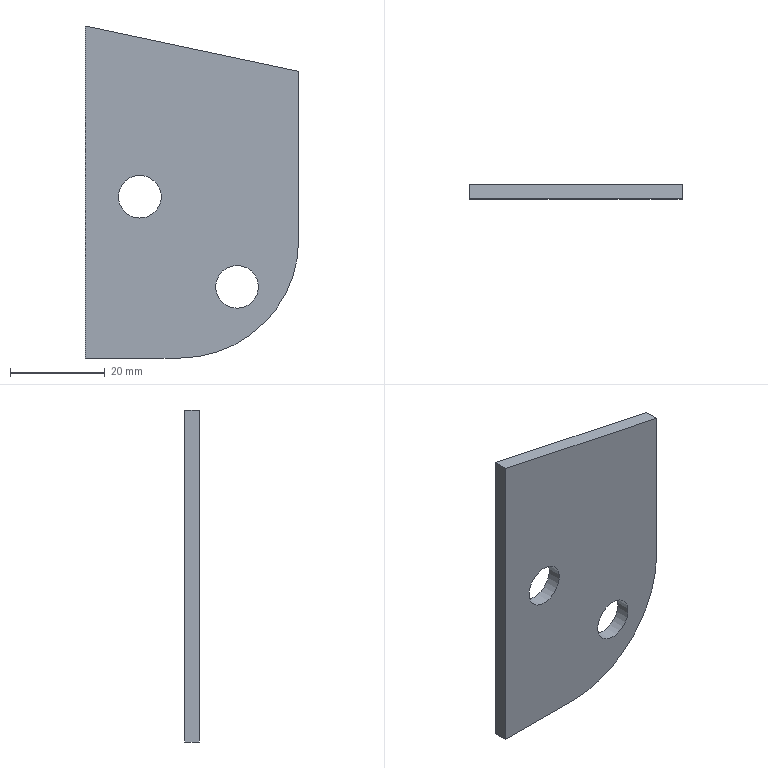Part | STEP file | 5091203 | 1 solid | 9 faces | box 45 x 3 x 70 mm | volume 8020 mm3 | plane 6 | cylinder 3 | commonest cylinder face diameters 9 x2 50 x1
STEP:
#1=CARTESIAN_POINT('',(0.,0.,0.));
#2=DIRECTION('',(0.,0.,1.));
#3=DIRECTION('',(1.,0.,0.));
#4=AXIS2_PLACEMENT_3D('',#1,#2,#3);
#5=CARTESIAN_POINT('',(22.5,1.5,25.435));
#6=VERTEX_POINT('',#5);
#7=CARTESIAN_POINT('',(22.5,1.5,-10.));
#8=VERTEX_POINT('',#7);
#9=CARTESIAN_POINT('',(22.5,1.5,35.));
#10=DIRECTION('',(0.,0.,-1.));
#11=VECTOR('',#10,1.);
#12=LINE('',#9,#11);
#13=CARTESIAN_POINT('',(22.5,1.5,35.));
#14=DIRECTION('',(-1.,0.,0.));
#15=DIRECTION('',(0.,0.,1.));
#16=AXIS2_PLACEMENT_3D('',#13,#14,#15);
#17=PLANE('',#16);
#18=CARTESIAN_POINT('',(0.,0.));
#19=DIRECTION('',(-1.,0.));
#20=VECTOR('',#19,1.);
#21=LINE('',#18,#20);
#22=(GEOMETRIC_REPRESENTATION_CONTEXT(2)PARAMETRIC_REPRESENTATION_CONTEXT()REPRESENTATION_CONTEXT('',''));
#23=DEFINITIONAL_REPRESENTATION('',(#21),#22);
#24=PCURVE('',#17,#23);
#25=CARTESIAN_POINT('',(-22.5,1.5,35.));
#26=DIRECTION('',(0.,-1.,0.));
#27=DIRECTION('',(0.,0.,-1.));
#28=AXIS2_PLACEMENT_3D('',#25,#26,#27);
#29=PLANE('',#28);
#30=CARTESIAN_POINT('',(0.,45.));
#31=DIRECTION('',(1.,0.));
#32=VECTOR('',#31,1.);
#33=LINE('',#30,#32);
#34=(GEOMETRIC_REPRESENTATION_CONTEXT(2)PARAMETRIC_REPRESENTATION_CONTEXT()REPRESENTATION_CONTEXT('',''));
#35=DEFINITIONAL_REPRESENTATION('',(#33),#34);
#36=PCURVE('',#29,#35);
#37=SURFACE_CURVE('',#12,(#24,#36),.PCURVE_S1.);
#38=EDGE_CURVE('',#6,#8,#37,.T.);
#39=ORIENTED_EDGE('',*,*,#38,.F.);
#40=CARTESIAN_POINT('',(22.5,-1.5,25.435));
#41=VERTEX_POINT('',#40);
#42=CARTESIAN_POINT('',(22.5,1.5,25.435));
#43=DIRECTION('',(0.,-1.,0.));
#44=VECTOR('',#43,1.);
#45=LINE('',#42,#44);
#46=CARTESIAN_POINT('',(-9.565,0.));
#47=DIRECTION('',(0.,-1.));
#48=VECTOR('',#47,1.);
#49=LINE('',#46,#48);
#50=(GEOMETRIC_REPRESENTATION_CONTEXT(2)PARAMETRIC_REPRESENTATION_CONTEXT()REPRESENTATION_CONTEXT('',''));
#51=DEFINITIONAL_REPRESENTATION('',(#49),#50);
#52=PCURVE('',#17,#51);
#53=CARTESIAN_POINT('',(-22.5,109.338,35.));
#54=DIRECTION('',(-0.2079,0.,-0.9781));
#55=DIRECTION('',(-0.9781,0.,0.2079));
#56=AXIS2_PLACEMENT_3D('',#53,#54,#55);
#57=PLANE('',#56);
#58=CARTESIAN_POINT('',(-46.005,-107.838));
#59=DIRECTION('',(0.,-1.));
#60=VECTOR('',#59,1.);
#61=LINE('',#58,#60);
#62=(GEOMETRIC_REPRESENTATION_CONTEXT(2)PARAMETRIC_REPRESENTATION_CONTEXT()REPRESENTATION_CONTEXT('',''));
#63=DEFINITIONAL_REPRESENTATION('',(#61),#62);
#64=PCURVE('',#57,#63);
#65=SURFACE_CURVE('',#45,(#52,#64),.PCURVE_S1.);
#66=EDGE_CURVE('',#6,#41,#65,.T.);
#67=ORIENTED_EDGE('',*,*,#66,.T.);
#68=CARTESIAN_POINT('',(22.5,-1.5,-10.));
#69=VERTEX_POINT('',#68);
#70=CARTESIAN_POINT('',(22.5,-1.5,35.));
#71=DIRECTION('',(0.,0.,-1.));
#72=VECTOR('',#71,1.);
#73=LINE('',#70,#72);
#74=CARTESIAN_POINT('',(0.,-3.));
#75=DIRECTION('',(-1.,0.));
#76=VECTOR('',#75,1.);
#77=LINE('',#74,#76);
#78=(GEOMETRIC_REPRESENTATION_CONTEXT(2)PARAMETRIC_REPRESENTATION_CONTEXT()REPRESENTATION_CONTEXT('',''));
#79=DEFINITIONAL_REPRESENTATION('',(#77),#78);
#80=PCURVE('',#17,#79);
#81=CARTESIAN_POINT('',(-22.5,-1.5,35.));
#82=DIRECTION('',(0.,1.,0.));
#83=DIRECTION('',(0.,0.,1.));
#84=AXIS2_PLACEMENT_3D('',#81,#82,#83);
#85=PLANE('',#84);
#86=CARTESIAN_POINT('',(0.,45.));
#87=DIRECTION('',(-1.,0.));
#88=VECTOR('',#87,1.);
#89=LINE('',#86,#88);
#90=(GEOMETRIC_REPRESENTATION_CONTEXT(2)PARAMETRIC_REPRESENTATION_CONTEXT()REPRESENTATION_CONTEXT('',''));
#91=DEFINITIONAL_REPRESENTATION('',(#89),#90);
#92=PCURVE('',#85,#91);
#93=SURFACE_CURVE('',#73,(#80,#92),.PCURVE_S1.);
#94=EDGE_CURVE('',#41,#69,#93,.T.);
#95=ORIENTED_EDGE('',*,*,#94,.T.);
#96=CARTESIAN_POINT('',(22.5,1.5,-10.));
#97=DIRECTION('',(0.,1.,0.));
#98=VECTOR('',#97,1.);
#99=LINE('',#96,#98);
#100=CARTESIAN_POINT('',(-45.,0.));
#101=DIRECTION('',(0.,1.));
#102=VECTOR('',#101,1.);
#103=LINE('',#100,#102);
#104=(GEOMETRIC_REPRESENTATION_CONTEXT(2)PARAMETRIC_REPRESENTATION_CONTEXT()REPRESENTATION_CONTEXT('',''));
#105=DEFINITIONAL_REPRESENTATION('',(#103),#104);
#106=PCURVE('',#17,#105);
#107=CARTESIAN_POINT('',(-2.5,1.5,-10.));
#108=DIRECTION('',(0.,1.,0.));
#109=DIRECTION('',(0.,0.,1.));
#110=AXIS2_PLACEMENT_3D('',#107,#108,#109);
#111=CYLINDRICAL_SURFACE('',#110,25.);
#112=CARTESIAN_POINT('',(1.571,0.));
#113=DIRECTION('',(0.,1.));
#114=VECTOR('',#113,1.);
#115=LINE('',#112,#114);
#116=(GEOMETRIC_REPRESENTATION_CONTEXT(2)PARAMETRIC_REPRESENTATION_CONTEXT()REPRESENTATION_CONTEXT('',''));
#117=DEFINITIONAL_REPRESENTATION('',(#115),#116);
#118=PCURVE('',#111,#117);
#119=SURFACE_CURVE('',#99,(#106,#118),.PCURVE_S1.);
#120=EDGE_CURVE('',#69,#8,#119,.T.);
#121=ORIENTED_EDGE('',*,*,#120,.T.);
#122=EDGE_LOOP('',(#39,#67,#95,#121));
#123=FACE_BOUND('',#122,.T.);
#124=ADVANCED_FACE('',(#123),#17,.F.);
#125=CARTESIAN_POINT('',(9.5,1.5,-15.5));
#126=VERTEX_POINT('',#125);
#127=CARTESIAN_POINT('',(9.5,1.5,-20.));
#128=DIRECTION('',(0.,1.,0.));
#129=DIRECTION('',(0.,0.,1.));
#130=AXIS2_PLACEMENT_3D('',#127,#128,#129);
#131=CIRCLE('',#130,4.5);
#132=CARTESIAN_POINT('',(50.5,32.));
#133=CARTESIAN_POINT('',(50.5,39.794));
#134=CARTESIAN_POINT('',(57.25,35.897));
#135=CARTESIAN_POINT('',(64.,32.));
#136=CARTESIAN_POINT('',(57.25,28.103));
#137=CARTESIAN_POINT('',(50.5,24.206));
#138=CARTESIAN_POINT('',(50.5,32.));
#139=(BOUNDED_CURVE()B_SPLINE_CURVE(2,(#132,#133,#134,#135,#136,#137,#138),.UNSPECIFIED.,.T.,.F.)B_SPLINE_CURVE_WITH_KNOTS((1,2,2,2,2,1),(-2.094,0.,2.094,4.189,6.283,8.378),.UNSPECIFIED.)CURVE()GEOMETRIC_REPRESENTATION_ITEM()RATIONAL_B_SPLINE_CURVE((1.,0.5,1.,0.5,1.,0.5,1.))REPRESENTATION_ITEM(''));
#140=(GEOMETRIC_REPRESENTATION_CONTEXT(2)PARAMETRIC_REPRESENTATION_CONTEXT()REPRESENTATION_CONTEXT('',''));
#141=DEFINITIONAL_REPRESENTATION('',(#139),#140);
#142=PCURVE('',#29,#141);
#143=CARTESIAN_POINT('',(9.5,-8.5,-20.));
#144=DIRECTION('',(0.,1.,0.));
#145=DIRECTION('',(0.,0.,1.));
#146=AXIS2_PLACEMENT_3D('',#143,#144,#145);
#147=CYLINDRICAL_SURFACE('',#146,4.5);
#148=CARTESIAN_POINT('',(0.,10.));
#149=DIRECTION('',(1.,0.));
#150=VECTOR('',#149,1.);
#151=LINE('',#148,#150);
#152=(GEOMETRIC_REPRESENTATION_CONTEXT(2)PARAMETRIC_REPRESENTATION_CONTEXT()REPRESENTATION_CONTEXT('',''));
#153=DEFINITIONAL_REPRESENTATION('',(#151),#152);
#154=PCURVE('',#147,#153);
#155=SURFACE_CURVE('',#131,(#142,#154),.PCURVE_S1.);
#156=EDGE_CURVE('',#126,#126,#155,.T.);
#157=ORIENTED_EDGE('',*,*,#156,.F.);
#158=EDGE_LOOP('',(#157));
#159=FACE_BOUND('',#158,.T.);
#160=CARTESIAN_POINT('',(-11.,1.5,3.5));
#161=VERTEX_POINT('',#160);
#162=CARTESIAN_POINT('',(-11.,1.5,-1.));
#163=DIRECTION('',(0.,1.,0.));
#164=DIRECTION('',(0.,0.,1.));
#165=AXIS2_PLACEMENT_3D('',#162,#163,#164);
#166=CIRCLE('',#165,4.5);
#167=CARTESIAN_POINT('',(31.5,11.5));
#168=CARTESIAN_POINT('',(31.5,19.294));
#169=CARTESIAN_POINT('',(38.25,15.397));
#170=CARTESIAN_POINT('',(45.,11.5));
#171=CARTESIAN_POINT('',(38.25,7.603));
#172=CARTESIAN_POINT('',(31.5,3.706));
#173=CARTESIAN_POINT('',(31.5,11.5));
#174=(BOUNDED_CURVE()B_SPLINE_CURVE(2,(#167,#168,#169,#170,#171,#172,#173),.UNSPECIFIED.,.T.,.F.)B_SPLINE_CURVE_WITH_KNOTS((1,2,2,2,2,1),(-2.094,0.,2.094,4.189,6.283,8.378),.UNSPECIFIED.)CURVE()GEOMETRIC_REPRESENTATION_ITEM()RATIONAL_B_SPLINE_CURVE((1.,0.5,1.,0.5,1.,0.5,1.))REPRESENTATION_ITEM(''));
#175=(GEOMETRIC_REPRESENTATION_CONTEXT(2)PARAMETRIC_REPRESENTATION_CONTEXT()REPRESENTATION_CONTEXT('',''));
#176=DEFINITIONAL_REPRESENTATION('',(#174),#175);
#177=PCURVE('',#29,#176);
#178=CARTESIAN_POINT('',(-11.,-8.5,-1.));
#179=DIRECTION('',(0.,1.,0.));
#180=DIRECTION('',(0.,0.,1.));
#181=AXIS2_PLACEMENT_3D('',#178,#179,#180);
#182=CYLINDRICAL_SURFACE('',#181,4.5);
#183=CARTESIAN_POINT('',(0.,10.));
#184=DIRECTION('',(1.,0.));
#185=VECTOR('',#184,1.);
#186=LINE('',#183,#185);
#187=(GEOMETRIC_REPRESENTATION_CONTEXT(2)PARAMETRIC_REPRESENTATION_CONTEXT()REPRESENTATION_CONTEXT('',''));
#188=DEFINITIONAL_REPRESENTATION('',(#186),#187);
#189=PCURVE('',#182,#188);
#190=SURFACE_CURVE('',#166,(#177,#189),.PCURVE_S1.);
#191=EDGE_CURVE('',#161,#161,#190,.T.);
#192=ORIENTED_EDGE('',*,*,#191,.F.);
#193=EDGE_LOOP('',(#192));
#194=FACE_BOUND('',#193,.T.);
#195=CARTESIAN_POINT('',(-22.5,1.5,35.));
#196=VERTEX_POINT('',#195);
#197=CARTESIAN_POINT('',(-22.5,1.5,-35.));
#198=VERTEX_POINT('',#197);
#199=CARTESIAN_POINT('',(-22.5,1.5,35.));
#200=DIRECTION('',(0.,0.,-1.));
#201=VECTOR('',#200,1.);
#202=LINE('',#199,#201);
#203=CARTESIAN_POINT('',(0.,0.));
#204=DIRECTION('',(1.,0.));
#205=VECTOR('',#204,1.);
#206=LINE('',#203,#205);
#207=(GEOMETRIC_REPRESENTATION_CONTEXT(2)PARAMETRIC_REPRESENTATION_CONTEXT()REPRESENTATION_CONTEXT('',''));
#208=DEFINITIONAL_REPRESENTATION('',(#206),#207);
#209=PCURVE('',#29,#208);
#210=CARTESIAN_POINT('',(-22.5,1.5,35.));
#211=DIRECTION('',(1.,0.,0.));
#212=DIRECTION('',(0.,0.,-1.));
#213=AXIS2_PLACEMENT_3D('',#210,#211,#212);
#214=PLANE('',#213);
#215=CARTESIAN_POINT('',(0.,0.));
#216=DIRECTION('',(1.,0.));
#217=VECTOR('',#216,1.);
#218=LINE('',#215,#217);
#219=(GEOMETRIC_REPRESENTATION_CONTEXT(2)PARAMETRIC_REPRESENTATION_CONTEXT()REPRESENTATION_CONTEXT('',''));
#220=DEFINITIONAL_REPRESENTATION('',(#218),#219);
#221=PCURVE('',#214,#220);
#222=SURFACE_CURVE('',#202,(#209,#221),.PCURVE_S1.);
#223=EDGE_CURVE('',#196,#198,#222,.T.);
#224=ORIENTED_EDGE('',*,*,#223,.F.);
#225=CARTESIAN_POINT('',(-22.5,1.5,35.));
#226=DIRECTION('',(0.9781,0.,-0.2079));
#227=VECTOR('',#226,1.);
#228=LINE('',#225,#227);
#229=CARTESIAN_POINT('',(0.,0.));
#230=DIRECTION('',(0.2079,0.9781));
#231=VECTOR('',#230,1.);
#232=LINE('',#229,#231);
#233=(GEOMETRIC_REPRESENTATION_CONTEXT(2)PARAMETRIC_REPRESENTATION_CONTEXT()REPRESENTATION_CONTEXT('',''));
#234=DEFINITIONAL_REPRESENTATION('',(#232),#233);
#235=PCURVE('',#29,#234);
#236=CARTESIAN_POINT('',(0.,-107.838));
#237=DIRECTION('',(-1.,0.));
#238=VECTOR('',#237,1.);
#239=LINE('',#236,#238);
#240=(GEOMETRIC_REPRESENTATION_CONTEXT(2)PARAMETRIC_REPRESENTATION_CONTEXT()REPRESENTATION_CONTEXT('',''));
#241=DEFINITIONAL_REPRESENTATION('',(#239),#240);
#242=PCURVE('',#57,#241);
#243=SURFACE_CURVE('',#228,(#235,#242),.PCURVE_S1.);
#244=EDGE_CURVE('',#196,#6,#243,.T.);
#245=ORIENTED_EDGE('',*,*,#244,.T.);
#246=ORIENTED_EDGE('',*,*,#38,.T.);
#247=CARTESIAN_POINT('',(-2.5,1.5,-35.));
#248=VERTEX_POINT('',#247);
#249=CARTESIAN_POINT('',(-2.5,1.5,-10.));
#250=DIRECTION('',(0.,1.,0.));
#251=DIRECTION('',(0.,0.,-1.));
#252=AXIS2_PLACEMENT_3D('',#249,#250,#251);
#253=CIRCLE('',#252,25.);
#254=CARTESIAN_POINT('',(70.,20.));
#255=CARTESIAN_POINT('',(70.,-23.301));
#256=CARTESIAN_POINT('',(32.5,-1.651));
#257=CARTESIAN_POINT('',(-5.,20.));
#258=CARTESIAN_POINT('',(32.5,41.651));
#259=CARTESIAN_POINT('',(70.,63.301));
#260=CARTESIAN_POINT('',(70.,20.));
#261=(BOUNDED_CURVE()B_SPLINE_CURVE(2,(#254,#255,#256,#257,#258,#259,#260),.UNSPECIFIED.,.T.,.F.)B_SPLINE_CURVE_WITH_KNOTS((1,2,2,2,2,1),(-2.094,0.,2.094,4.189,6.283,8.378),.UNSPECIFIED.)CURVE()GEOMETRIC_REPRESENTATION_ITEM()RATIONAL_B_SPLINE_CURVE((1.,0.5,1.,0.5,1.,0.5,1.))REPRESENTATION_ITEM(''));
#262=(GEOMETRIC_REPRESENTATION_CONTEXT(2)PARAMETRIC_REPRESENTATION_CONTEXT()REPRESENTATION_CONTEXT('',''));
#263=DEFINITIONAL_REPRESENTATION('',(#261),#262);
#264=PCURVE('',#29,#263);
#265=CARTESIAN_POINT('',(-3.142,0.));
#266=DIRECTION('',(1.,0.));
#267=VECTOR('',#266,1.);
#268=LINE('',#265,#267);
#269=(GEOMETRIC_REPRESENTATION_CONTEXT(2)PARAMETRIC_REPRESENTATION_CONTEXT()REPRESENTATION_CONTEXT('',''));
#270=DEFINITIONAL_REPRESENTATION('',(#268),#269);
#271=PCURVE('',#111,#270);
#272=SURFACE_CURVE('',#253,(#264,#271),.PCURVE_S1.);
#273=EDGE_CURVE('',#8,#248,#272,.T.);
#274=ORIENTED_EDGE('',*,*,#273,.T.);
#275=CARTESIAN_POINT('',(-22.5,1.5,-35.));
#276=DIRECTION('',(-1.,0.,0.));
#277=VECTOR('',#276,1.);
#278=LINE('',#275,#277);
#279=CARTESIAN_POINT('',(70.,0.));
#280=DIRECTION('',(0.,-1.));
#281=VECTOR('',#280,1.);
#282=LINE('',#279,#281);
#283=(GEOMETRIC_REPRESENTATION_CONTEXT(2)PARAMETRIC_REPRESENTATION_CONTEXT()REPRESENTATION_CONTEXT('',''));
#284=DEFINITIONAL_REPRESENTATION('',(#282),#283);
#285=PCURVE('',#29,#284);
#286=CARTESIAN_POINT('',(0.,0.,-35.));
#287=DIRECTION('',(0.,0.,1.));
#288=DIRECTION('',(1.,0.,0.));
#289=AXIS2_PLACEMENT_3D('',#286,#287,#288);
#290=PLANE('',#289);
#291=CARTESIAN_POINT('',(-22.5,1.5));
#292=DIRECTION('',(-1.,0.));
#293=VECTOR('',#292,1.);
#294=LINE('',#291,#293);
#295=(GEOMETRIC_REPRESENTATION_CONTEXT(2)PARAMETRIC_REPRESENTATION_CONTEXT()REPRESENTATION_CONTEXT('',''));
#296=DEFINITIONAL_REPRESENTATION('',(#294),#295);
#297=PCURVE('',#290,#296);
#298=SURFACE_CURVE('',#278,(#285,#297),.PCURVE_S1.);
#299=EDGE_CURVE('',#248,#198,#298,.T.);
#300=ORIENTED_EDGE('',*,*,#299,.T.);
#301=EDGE_LOOP('',(#224,#245,#246,#274,#300));
#302=FACE_BOUND('',#301,.T.);
#303=ADVANCED_FACE('',(#159,#194,#302),#29,.F.);
#304=CARTESIAN_POINT('',(-22.5,-1.5,-35.));
#305=VERTEX_POINT('',#304);
#306=CARTESIAN_POINT('',(-22.5,1.5,-35.));
#307=DIRECTION('',(0.,-1.,0.));
#308=VECTOR('',#307,1.);
#309=LINE('',#306,#308);
#310=CARTESIAN_POINT('',(70.,0.));
#311=DIRECTION('',(0.,-1.));
#312=VECTOR('',#311,1.);
#313=LINE('',#310,#312);
#314=(GEOMETRIC_REPRESENTATION_CONTEXT(2)PARAMETRIC_REPRESENTATION_CONTEXT()REPRESENTATION_CONTEXT('',''));
#315=DEFINITIONAL_REPRESENTATION('',(#313),#314);
#316=PCURVE('',#214,#315);
#317=CARTESIAN_POINT('',(-22.5,1.5));
#318=DIRECTION('',(0.,-1.));
#319=VECTOR('',#318,1.);
#320=LINE('',#317,#319);
#321=(GEOMETRIC_REPRESENTATION_CONTEXT(2)PARAMETRIC_REPRESENTATION_CONTEXT()REPRESENTATION_CONTEXT('',''));
#322=DEFINITIONAL_REPRESENTATION('',(#320),#321);
#323=PCURVE('',#290,#322);
#324=SURFACE_CURVE('',#309,(#316,#323),.PCURVE_S1.);
#325=EDGE_CURVE('',#198,#305,#324,.T.);
#326=ORIENTED_EDGE('',*,*,#325,.T.);
#327=CARTESIAN_POINT('',(-22.5,-1.5,35.));
#328=VERTEX_POINT('',#327);
#329=CARTESIAN_POINT('',(-22.5,-1.5,35.));
#330=DIRECTION('',(0.,0.,-1.));
#331=VECTOR('',#330,1.);
#332=LINE('',#329,#331);
#333=CARTESIAN_POINT('',(0.,-3.));
#334=DIRECTION('',(1.,0.));
#335=VECTOR('',#334,1.);
#336=LINE('',#333,#335);
#337=(GEOMETRIC_REPRESENTATION_CONTEXT(2)PARAMETRIC_REPRESENTATION_CONTEXT()REPRESENTATION_CONTEXT('',''));
#338=DEFINITIONAL_REPRESENTATION('',(#336),#337);
#339=PCURVE('',#214,#338);
#340=CARTESIAN_POINT('',(0.,0.));
#341=DIRECTION('',(-1.,0.));
#342=VECTOR('',#341,1.);
#343=LINE('',#340,#342);
#344=(GEOMETRIC_REPRESENTATION_CONTEXT(2)PARAMETRIC_REPRESENTATION_CONTEXT()REPRESENTATION_CONTEXT('',''));
#345=DEFINITIONAL_REPRESENTATION('',(#343),#344);
#346=PCURVE('',#85,#345);
#347=SURFACE_CURVE('',#332,(#339,#346),.PCURVE_S1.);
#348=EDGE_CURVE('',#328,#305,#347,.T.);
#349=ORIENTED_EDGE('',*,*,#348,.F.);
#350=CARTESIAN_POINT('',(-22.5,1.5,35.));
#351=DIRECTION('',(0.,-1.,0.));
#352=VECTOR('',#351,1.);
#353=LINE('',#350,#352);
#354=CARTESIAN_POINT('',(0.,0.));
#355=DIRECTION('',(0.,-1.));
#356=VECTOR('',#355,1.);
#357=LINE('',#354,#356);
#358=(GEOMETRIC_REPRESENTATION_CONTEXT(2)PARAMETRIC_REPRESENTATION_CONTEXT()REPRESENTATION_CONTEXT('',''));
#359=DEFINITIONAL_REPRESENTATION('',(#357),#358);
#360=PCURVE('',#214,#359);
#361=CARTESIAN_POINT('',(0.,-107.838));
#362=DIRECTION('',(0.,-1.));
#363=VECTOR('',#362,1.);
#364=LINE('',#361,#363);
#365=(GEOMETRIC_REPRESENTATION_CONTEXT(2)PARAMETRIC_REPRESENTATION_CONTEXT()REPRESENTATION_CONTEXT('',''));
#366=DEFINITIONAL_REPRESENTATION('',(#364),#365);
#367=PCURVE('',#57,#366);
#368=SURFACE_CURVE('',#353,(#360,#367),.PCURVE_S1.);
#369=EDGE_CURVE('',#196,#328,#368,.T.);
#370=ORIENTED_EDGE('',*,*,#369,.F.);
#371=ORIENTED_EDGE('',*,*,#223,.T.);
#372=EDGE_LOOP('',(#326,#349,#370,#371));
#373=FACE_BOUND('',#372,.T.);
#374=ADVANCED_FACE('',(#373),#214,.F.);
#375=CARTESIAN_POINT('',(9.5,-1.5,-15.5));
#376=VERTEX_POINT('',#375);
#377=CARTESIAN_POINT('',(9.5,-1.5,-20.));
#378=DIRECTION('',(0.,1.,0.));
#379=DIRECTION('',(0.,0.,1.));
#380=AXIS2_PLACEMENT_3D('',#377,#378,#379);
#381=CIRCLE('',#380,4.5);
#382=CARTESIAN_POINT('',(-55.,32.));
#383=DIRECTION('',(1.,0.));
#384=AXIS2_PLACEMENT_2D('',#382,#383);
#385=CIRCLE('',#384,4.5);
#386=(GEOMETRIC_REPRESENTATION_CONTEXT(2)PARAMETRIC_REPRESENTATION_CONTEXT()REPRESENTATION_CONTEXT('',''));
#387=DEFINITIONAL_REPRESENTATION('',(#385),#386);
#388=PCURVE('',#85,#387);
#389=CARTESIAN_POINT('',(0.,7.));
#390=DIRECTION('',(1.,0.));
#391=VECTOR('',#390,1.);
#392=LINE('',#389,#391);
#393=(GEOMETRIC_REPRESENTATION_CONTEXT(2)PARAMETRIC_REPRESENTATION_CONTEXT()REPRESENTATION_CONTEXT('',''));
#394=DEFINITIONAL_REPRESENTATION('',(#392),#393);
#395=PCURVE('',#147,#394);
#396=SURFACE_CURVE('',#381,(#388,#395),.PCURVE_S1.);
#397=EDGE_CURVE('',#376,#376,#396,.T.);
#398=ORIENTED_EDGE('',*,*,#397,.T.);
#399=EDGE_LOOP('',(#398));
#400=FACE_BOUND('',#399,.T.);
#401=CARTESIAN_POINT('',(-11.,-1.5,3.5));
#402=VERTEX_POINT('',#401);
#403=CARTESIAN_POINT('',(-11.,-1.5,-1.));
#404=DIRECTION('',(0.,1.,0.));
#405=DIRECTION('',(0.,0.,1.));
#406=AXIS2_PLACEMENT_3D('',#403,#404,#405);
#407=CIRCLE('',#406,4.5);
#408=CARTESIAN_POINT('',(-36.,11.5));
#409=DIRECTION('',(1.,0.));
#410=AXIS2_PLACEMENT_2D('',#408,#409);
#411=CIRCLE('',#410,4.5);
#412=(GEOMETRIC_REPRESENTATION_CONTEXT(2)PARAMETRIC_REPRESENTATION_CONTEXT()REPRESENTATION_CONTEXT('',''));
#413=DEFINITIONAL_REPRESENTATION('',(#411),#412);
#414=PCURVE('',#85,#413);
#415=CARTESIAN_POINT('',(0.,7.));
#416=DIRECTION('',(1.,0.));
#417=VECTOR('',#416,1.);
#418=LINE('',#415,#417);
#419=(GEOMETRIC_REPRESENTATION_CONTEXT(2)PARAMETRIC_REPRESENTATION_CONTEXT()REPRESENTATION_CONTEXT('',''));
#420=DEFINITIONAL_REPRESENTATION('',(#418),#419);
#421=PCURVE('',#182,#420);
#422=SURFACE_CURVE('',#407,(#414,#421),.PCURVE_S1.);
#423=EDGE_CURVE('',#402,#402,#422,.T.);
#424=ORIENTED_EDGE('',*,*,#423,.T.);
#425=EDGE_LOOP('',(#424));
#426=FACE_BOUND('',#425,.T.);
#427=ORIENTED_EDGE('',*,*,#94,.F.);
#428=CARTESIAN_POINT('',(-22.5,-1.5,35.));
#429=DIRECTION('',(-0.9781,0.,0.2079));
#430=VECTOR('',#429,1.);
#431=LINE('',#428,#430);
#432=CARTESIAN_POINT('',(0.,0.));
#433=DIRECTION('',(0.2079,-0.9781));
#434=VECTOR('',#433,1.);
#435=LINE('',#432,#434);
#436=(GEOMETRIC_REPRESENTATION_CONTEXT(2)PARAMETRIC_REPRESENTATION_CONTEXT()REPRESENTATION_CONTEXT('',''));
#437=DEFINITIONAL_REPRESENTATION('',(#435),#436);
#438=PCURVE('',#85,#437);
#439=CARTESIAN_POINT('',(0.,-110.838));
#440=DIRECTION('',(1.,0.));
#441=VECTOR('',#440,1.);
#442=LINE('',#439,#441);
#443=(GEOMETRIC_REPRESENTATION_CONTEXT(2)PARAMETRIC_REPRESENTATION_CONTEXT()REPRESENTATION_CONTEXT('',''));
#444=DEFINITIONAL_REPRESENTATION('',(#442),#443);
#445=PCURVE('',#57,#444);
#446=SURFACE_CURVE('',#431,(#438,#445),.PCURVE_S1.);
#447=EDGE_CURVE('',#41,#328,#446,.T.);
#448=ORIENTED_EDGE('',*,*,#447,.T.);
#449=ORIENTED_EDGE('',*,*,#348,.T.);
#450=CARTESIAN_POINT('',(-2.5,-1.5,-35.));
#451=VERTEX_POINT('',#450);
#452=CARTESIAN_POINT('',(-22.5,-1.5,-35.));
#453=DIRECTION('',(1.,0.,0.));
#454=VECTOR('',#453,1.);
#455=LINE('',#452,#454);
#456=CARTESIAN_POINT('',(-70.,0.));
#457=DIRECTION('',(0.,1.));
#458=VECTOR('',#457,1.);
#459=LINE('',#456,#458);
#460=(GEOMETRIC_REPRESENTATION_CONTEXT(2)PARAMETRIC_REPRESENTATION_CONTEXT()REPRESENTATION_CONTEXT('',''));
#461=DEFINITIONAL_REPRESENTATION('',(#459),#460);
#462=PCURVE('',#85,#461);
#463=CARTESIAN_POINT('',(-22.5,-1.5));
#464=DIRECTION('',(1.,0.));
#465=VECTOR('',#464,1.);
#466=LINE('',#463,#465);
#467=(GEOMETRIC_REPRESENTATION_CONTEXT(2)PARAMETRIC_REPRESENTATION_CONTEXT()REPRESENTATION_CONTEXT('',''));
#468=DEFINITIONAL_REPRESENTATION('',(#466),#467);
#469=PCURVE('',#290,#468);
#470=SURFACE_CURVE('',#455,(#462,#469),.PCURVE_S1.);
#471=EDGE_CURVE('',#305,#451,#470,.T.);
#472=ORIENTED_EDGE('',*,*,#471,.T.);
#473=CARTESIAN_POINT('',(-2.5,-1.5,-10.));
#474=DIRECTION('',(0.,-1.,0.));
#475=DIRECTION('',(0.,0.,1.));
#476=AXIS2_PLACEMENT_3D('',#473,#474,#475);
#477=CIRCLE('',#476,25.);
#478=CARTESIAN_POINT('',(-20.,20.));
#479=CARTESIAN_POINT('',(-20.,-23.301));
#480=CARTESIAN_POINT('',(-57.5,-1.651));
#481=CARTESIAN_POINT('',(-95.,20.));
#482=CARTESIAN_POINT('',(-57.5,41.651));
#483=CARTESIAN_POINT('',(-20.,63.301));
#484=CARTESIAN_POINT('',(-20.,20.));
#485=(BOUNDED_CURVE()B_SPLINE_CURVE(2,(#478,#479,#480,#481,#482,#483,#484),.UNSPECIFIED.,.T.,.F.)B_SPLINE_CURVE_WITH_KNOTS((1,2,2,2,2,1),(-2.094,0.,2.094,4.189,6.283,8.378),.UNSPECIFIED.)CURVE()GEOMETRIC_REPRESENTATION_ITEM()RATIONAL_B_SPLINE_CURVE((1.,0.5,1.,0.5,1.,0.5,1.))REPRESENTATION_ITEM(''));
#486=(GEOMETRIC_REPRESENTATION_CONTEXT(2)PARAMETRIC_REPRESENTATION_CONTEXT()REPRESENTATION_CONTEXT('',''));
#487=DEFINITIONAL_REPRESENTATION('',(#485),#486);
#488=PCURVE('',#85,#487);
#489=CARTESIAN_POINT('',(6.283,-3.));
#490=DIRECTION('',(-1.,0.));
#491=VECTOR('',#490,1.);
#492=LINE('',#489,#491);
#493=(GEOMETRIC_REPRESENTATION_CONTEXT(2)PARAMETRIC_REPRESENTATION_CONTEXT()REPRESENTATION_CONTEXT('',''));
#494=DEFINITIONAL_REPRESENTATION('',(#492),#493);
#495=PCURVE('',#111,#494);
#496=SURFACE_CURVE('',#477,(#488,#495),.PCURVE_S1.);
#497=EDGE_CURVE('',#451,#69,#496,.T.);
#498=ORIENTED_EDGE('',*,*,#497,.T.);
#499=EDGE_LOOP('',(#427,#448,#449,#472,#498));
#500=FACE_BOUND('',#499,.T.);
#501=ADVANCED_FACE('',(#400,#426,#500),#85,.F.);
#502=ORIENTED_EDGE('',*,*,#299,.F.);
#503=CARTESIAN_POINT('',(-2.5,0.,-35.));
#504=DIRECTION('',(0.,-1.,0.));
#505=VECTOR('',#504,1.);
#506=LINE('',#503,#505);
#507=CARTESIAN_POINT('',(-2.5,0.));
#508=DIRECTION('',(0.,-1.));
#509=VECTOR('',#508,1.);
#510=LINE('',#507,#509);
#511=(GEOMETRIC_REPRESENTATION_CONTEXT(2)PARAMETRIC_REPRESENTATION_CONTEXT()REPRESENTATION_CONTEXT('',''));
#512=DEFINITIONAL_REPRESENTATION('',(#510),#511);
#513=PCURVE('',#290,#512);
#514=CARTESIAN_POINT('',(3.142,-1.5));
#515=DIRECTION('',(0.,-1.));
#516=VECTOR('',#515,1.);
#517=LINE('',#514,#516);
#518=(GEOMETRIC_REPRESENTATION_CONTEXT(2)PARAMETRIC_REPRESENTATION_CONTEXT()REPRESENTATION_CONTEXT('',''));
#519=DEFINITIONAL_REPRESENTATION('',(#517),#518);
#520=PCURVE('',#111,#519);
#521=SURFACE_CURVE('',#506,(#513,#520),.PCURVE_S1.);
#522=EDGE_CURVE('',#248,#451,#521,.T.);
#523=ORIENTED_EDGE('',*,*,#522,.T.);
#524=ORIENTED_EDGE('',*,*,#471,.F.);
#525=ORIENTED_EDGE('',*,*,#325,.F.);
#526=EDGE_LOOP('',(#502,#523,#524,#525));
#527=FACE_BOUND('',#526,.T.);
#528=ADVANCED_FACE('',(#527),#290,.F.);
#529=ORIENTED_EDGE('',*,*,#497,.F.);
#530=ORIENTED_EDGE('',*,*,#522,.F.);
#531=ORIENTED_EDGE('',*,*,#273,.F.);
#532=ORIENTED_EDGE('',*,*,#120,.F.);
#533=EDGE_LOOP('',(#529,#530,#531,#532));
#534=FACE_BOUND('',#533,.T.);
#535=ADVANCED_FACE('',(#534),#111,.T.);
#536=ORIENTED_EDGE('',*,*,#244,.F.);
#537=ORIENTED_EDGE('',*,*,#369,.T.);
#538=ORIENTED_EDGE('',*,*,#447,.F.);
#539=ORIENTED_EDGE('',*,*,#66,.F.);
#540=EDGE_LOOP('',(#536,#537,#538,#539));
#541=FACE_BOUND('',#540,.T.);
#542=ADVANCED_FACE('',(#541),#57,.F.);
#543=ORIENTED_EDGE('',*,*,#191,.F.);
#544=CARTESIAN_POINT('',(-11.,-1.5,3.5));
#545=CARTESIAN_POINT('',(-11.,1.5,3.5));
#546=B_SPLINE_CURVE_WITH_KNOTS('',1,(#544,#545),.UNSPECIFIED.,.F.,.F.,(2,2),(7.,10.),.PIECEWISE_BEZIER_KNOTS.);
#547=CARTESIAN_POINT('',(0.,0.));
#548=DIRECTION('',(0.,1.));
#549=VECTOR('',#548,1.);
#550=LINE('',#547,#549);
#551=(GEOMETRIC_REPRESENTATION_CONTEXT(2)PARAMETRIC_REPRESENTATION_CONTEXT()REPRESENTATION_CONTEXT('',''));
#552=DEFINITIONAL_REPRESENTATION('',(#550),#551);
#553=PCURVE('',#182,#552);
#554=CARTESIAN_POINT('',(6.283,0.));
#555=DIRECTION('',(0.,1.));
#556=VECTOR('',#555,1.);
#557=LINE('',#554,#556);
#558=(GEOMETRIC_REPRESENTATION_CONTEXT(2)PARAMETRIC_REPRESENTATION_CONTEXT()REPRESENTATION_CONTEXT('',''));
#559=DEFINITIONAL_REPRESENTATION('',(#557),#558);
#560=PCURVE('',#182,#559);
#561=SEAM_CURVE('',#546,(#553,#560),.PCURVE_S1.);
#562=EDGE_CURVE('',#402,#161,#561,.T.);
#563=ORIENTED_EDGE('',*,*,#562,.F.);
#564=ORIENTED_EDGE('',*,*,#423,.T.);
#565=ORIENTED_EDGE('',*,*,#562,.T.);
#566=EDGE_LOOP('',(#543,#563,#564,#565));
#567=FACE_BOUND('',#566,.F.);
#568=ADVANCED_FACE('',(#567),#182,.F.);
#569=ORIENTED_EDGE('',*,*,#156,.F.);
#570=CARTESIAN_POINT('',(9.5,-1.5,-15.5));
#571=CARTESIAN_POINT('',(9.5,1.5,-15.5));
#572=B_SPLINE_CURVE_WITH_KNOTS('',1,(#570,#571),.UNSPECIFIED.,.F.,.F.,(2,2),(7.,10.),.PIECEWISE_BEZIER_KNOTS.);
#573=CARTESIAN_POINT('',(0.,0.));
#574=DIRECTION('',(0.,1.));
#575=VECTOR('',#574,1.);
#576=LINE('',#573,#575);
#577=(GEOMETRIC_REPRESENTATION_CONTEXT(2)PARAMETRIC_REPRESENTATION_CONTEXT()REPRESENTATION_CONTEXT('',''));
#578=DEFINITIONAL_REPRESENTATION('',(#576),#577);
#579=PCURVE('',#147,#578);
#580=CARTESIAN_POINT('',(6.283,0.));
#581=DIRECTION('',(0.,1.));
#582=VECTOR('',#581,1.);
#583=LINE('',#580,#582);
#584=(GEOMETRIC_REPRESENTATION_CONTEXT(2)PARAMETRIC_REPRESENTATION_CONTEXT()REPRESENTATION_CONTEXT('',''));
#585=DEFINITIONAL_REPRESENTATION('',(#583),#584);
#586=PCURVE('',#147,#585);
#587=SEAM_CURVE('',#572,(#579,#586),.PCURVE_S1.);
#588=EDGE_CURVE('',#376,#126,#587,.T.);
#589=ORIENTED_EDGE('',*,*,#588,.F.);
#590=ORIENTED_EDGE('',*,*,#397,.T.);
#591=ORIENTED_EDGE('',*,*,#588,.T.);
#592=EDGE_LOOP('',(#569,#589,#590,#591));
#593=FACE_BOUND('',#592,.F.);
#594=ADVANCED_FACE('',(#593),#147,.F.);
#595=CLOSED_SHELL('',(#124,#303,#374,#501,#528,#535,#542,#568,#594));
#596=MANIFOLD_SOLID_BREP('',#595);
#597=(LENGTH_UNIT()NAMED_UNIT(*)SI_UNIT(.MILLI.,.METRE.));
#598=UNCERTAINTY_MEASURE_WITH_UNIT(LENGTH_MEASURE(0.000002),#597,'','');
#599=(NAMED_UNIT(*)PLANE_ANGLE_UNIT()SI_UNIT($,.RADIAN.));
#600=(NAMED_UNIT(*)SI_UNIT($,.STERADIAN.)SOLID_ANGLE_UNIT());
#601=(GEOMETRIC_REPRESENTATION_CONTEXT(3)GLOBAL_UNCERTAINTY_ASSIGNED_CONTEXT((#598))GLOBAL_UNIT_ASSIGNED_CONTEXT((#597,#599,#600))REPRESENTATION_CONTEXT('',''));
#602=ADVANCED_BREP_SHAPE_REPRESENTATION('',(#4,#596),#601);